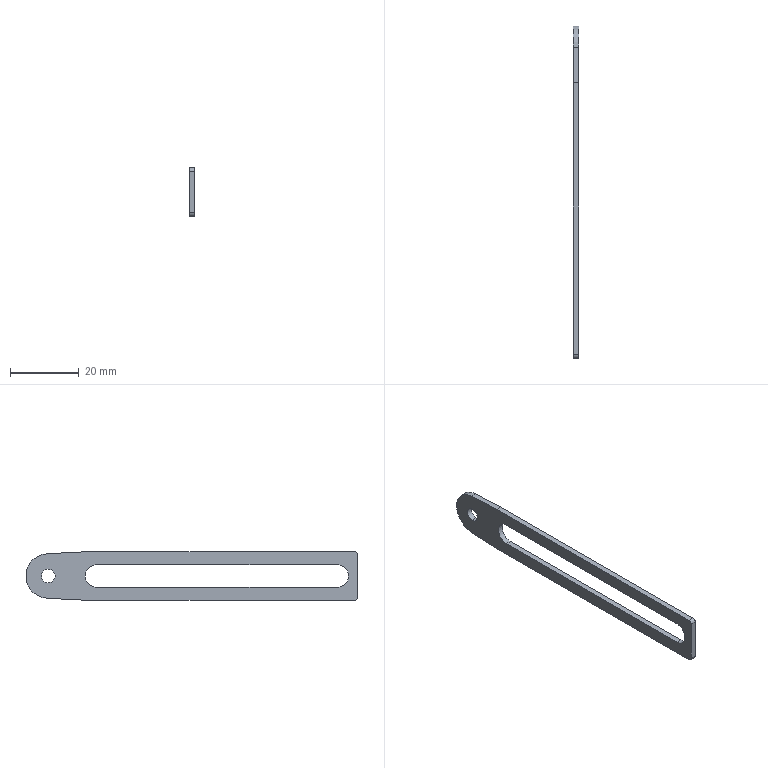Part | STEP file | Guide wheel mechanism revised.sldasm-Part-508 | 1 solid | 16 faces | box 1.6 x 96.5 x 14 mm | volume 1312 mm3 | plane 9 | cylinder 7 | commonest cylinder face diameters 2 x2 4 x2 6.5 x2 13 x1
STEP:
#1=CARTESIAN_POINT('',(0.,84.,-2.));
#2=VERTEX_POINT('',#1);
#3=CARTESIAN_POINT('',(0.,84.,2.));
#4=VERTEX_POINT('',#3);
#5=CARTESIAN_POINT('',(0.,84.,0.));
#6=DIRECTION('',(-1.,0.,0.));
#7=DIRECTION('',(0.,0.,-1.));
#8=AXIS2_PLACEMENT_3D('',#5,#6,#7);
#9=CIRCLE('',#8,2.);
#10=EDGE_CURVE('',#2,#4,#9,.T.);
#11=ORIENTED_EDGE('',*,*,#10,.T.);
#12=CARTESIAN_POINT('',(1.6,84.,2.));
#13=VERTEX_POINT('',#12);
#14=CARTESIAN_POINT('',(0.,84.,2.));
#15=DIRECTION('',(1.,0.,0.));
#16=VECTOR('',#15,1000.);
#17=LINE('',#14,#16);
#18=EDGE_CURVE('',#4,#13,#17,.T.);
#19=ORIENTED_EDGE('',*,*,#18,.T.);
#20=CARTESIAN_POINT('',(1.6,84.,-2.));
#21=VERTEX_POINT('',#20);
#22=CARTESIAN_POINT('',(1.6,84.,0.));
#23=DIRECTION('',(-1.,0.,0.));
#24=DIRECTION('',(0.,0.,-1.));
#25=AXIS2_PLACEMENT_3D('',#22,#23,#24);
#26=CIRCLE('',#25,2.);
#27=EDGE_CURVE('',#21,#13,#26,.T.);
#28=ORIENTED_EDGE('',*,*,#27,.F.);
#29=CARTESIAN_POINT('',(0.,84.,-2.));
#30=DIRECTION('',(1.,0.,0.));
#31=VECTOR('',#30,1000.);
#32=LINE('',#29,#31);
#33=EDGE_CURVE('',#2,#21,#32,.T.);
#34=ORIENTED_EDGE('',*,*,#33,.F.);
#35=EDGE_LOOP('',(#11,#19,#28,#34));
#36=FACE_OUTER_BOUND('',#35,.T.);
#37=CARTESIAN_POINT('',(0.,84.,0.));
#38=DIRECTION('',(1.,0.,0.));
#39=DIRECTION('',(0.,0.,-1.));
#40=AXIS2_PLACEMENT_3D('',#37,#38,#39);
#41=CYLINDRICAL_SURFACE('',#40,2.);
#42=ADVANCED_FACE('',(#36),#41,.F.);
#43=CARTESIAN_POINT('',(0.,70.,-3.25));
#44=VERTEX_POINT('',#43);
#45=CARTESIAN_POINT('',(0.,0.,-3.25));
#46=VERTEX_POINT('',#45);
#47=CARTESIAN_POINT('',(0.,0.,-3.25));
#48=DIRECTION('',(0.,-1.,0.));
#49=VECTOR('',#48,1000.);
#50=LINE('',#47,#49);
#51=EDGE_CURVE('',#44,#46,#50,.T.);
#52=ORIENTED_EDGE('',*,*,#51,.F.);
#53=CARTESIAN_POINT('',(0.,70.,3.25));
#54=VERTEX_POINT('',#53);
#55=CARTESIAN_POINT('',(0.,70.,0.));
#56=DIRECTION('',(-1.,0.,0.));
#57=DIRECTION('',(0.,0.,-1.));
#58=AXIS2_PLACEMENT_3D('',#55,#56,#57);
#59=CIRCLE('',#58,3.25);
#60=EDGE_CURVE('',#54,#44,#59,.T.);
#61=ORIENTED_EDGE('',*,*,#60,.F.);
#62=CARTESIAN_POINT('',(0.,0.,3.25));
#63=VERTEX_POINT('',#62);
#64=CARTESIAN_POINT('',(0.,0.,3.25));
#65=DIRECTION('',(0.,1.,0.));
#66=VECTOR('',#65,1000.);
#67=LINE('',#64,#66);
#68=EDGE_CURVE('',#63,#54,#67,.T.);
#69=ORIENTED_EDGE('',*,*,#68,.F.);
#70=CARTESIAN_POINT('',(0.,0.,0.));
#71=DIRECTION('',(-1.,0.,0.));
#72=DIRECTION('',(0.,0.,-1.));
#73=AXIS2_PLACEMENT_3D('',#70,#71,#72);
#74=CIRCLE('',#73,3.25);
#75=EDGE_CURVE('',#46,#63,#74,.T.);
#76=ORIENTED_EDGE('',*,*,#75,.F.);
#77=EDGE_LOOP('',(#52,#61,#69,#76));
#78=FACE_BOUND('',#77,.T.);
#79=ORIENTED_EDGE('',*,*,#10,.F.);
#80=CARTESIAN_POINT('',(0.,84.,0.));
#81=DIRECTION('',(-1.,0.,0.));
#82=DIRECTION('',(0.,0.,-1.));
#83=AXIS2_PLACEMENT_3D('',#80,#81,#82);
#84=CIRCLE('',#83,2.);
#85=EDGE_CURVE('',#4,#2,#84,.T.);
#86=ORIENTED_EDGE('',*,*,#85,.F.);
#87=EDGE_LOOP('',(#79,#86));
#88=FACE_BOUND('',#87,.T.);
#89=CARTESIAN_POINT('',(0.,84.32,6.492));
#90=VERTEX_POINT('',#89);
#91=CARTESIAN_POINT('',(0.,74.,7.));
#92=VERTEX_POINT('',#91);
#93=CARTESIAN_POINT('',(0.,84.32,6.492));
#94=DIRECTION('',(0.,-0.9988,0.04915));
#95=VECTOR('',#94,1000.);
#96=LINE('',#93,#95);
#97=EDGE_CURVE('',#90,#92,#96,.T.);
#98=ORIENTED_EDGE('',*,*,#97,.F.);
#99=CARTESIAN_POINT('',(0.,84.32,-6.492));
#100=VERTEX_POINT('',#99);
#101=CARTESIAN_POINT('',(0.,84.,0.));
#102=DIRECTION('',(1.,0.,0.));
#103=DIRECTION('',(0.,0.,-1.));
#104=AXIS2_PLACEMENT_3D('',#101,#102,#103);
#105=CIRCLE('',#104,6.5);
#106=EDGE_CURVE('',#100,#90,#105,.T.);
#107=ORIENTED_EDGE('',*,*,#106,.F.);
#108=CARTESIAN_POINT('',(0.,74.,-7.));
#109=VERTEX_POINT('',#108);
#110=CARTESIAN_POINT('',(0.,74.,-7.));
#111=DIRECTION('',(0.,0.9988,0.04915));
#112=VECTOR('',#111,1000.);
#113=LINE('',#110,#112);
#114=EDGE_CURVE('',#109,#100,#113,.T.);
#115=ORIENTED_EDGE('',*,*,#114,.F.);
#116=CARTESIAN_POINT('',(0.,-5.,-7.));
#117=VERTEX_POINT('',#116);
#118=CARTESIAN_POINT('',(0.,0.,-7.));
#119=DIRECTION('',(0.,1.,0.));
#120=VECTOR('',#119,1000.);
#121=LINE('',#118,#120);
#122=EDGE_CURVE('',#117,#109,#121,.T.);
#123=ORIENTED_EDGE('',*,*,#122,.F.);
#124=CARTESIAN_POINT('',(0.,-6.,-6.));
#125=VERTEX_POINT('',#124);
#126=CARTESIAN_POINT('',(0.,-5.,-6.));
#127=DIRECTION('',(1.,0.,0.));
#128=DIRECTION('',(0.,0.,1.));
#129=AXIS2_PLACEMENT_3D('',#126,#127,#128);
#130=CIRCLE('',#129,1.);
#131=EDGE_CURVE('',#125,#117,#130,.T.);
#132=ORIENTED_EDGE('',*,*,#131,.F.);
#133=CARTESIAN_POINT('',(0.,-6.,6.));
#134=VERTEX_POINT('',#133);
#135=CARTESIAN_POINT('',(0.,-6.,0.));
#136=DIRECTION('',(0.,0.,-1.));
#137=VECTOR('',#136,1000.);
#138=LINE('',#135,#137);
#139=EDGE_CURVE('',#134,#125,#138,.T.);
#140=ORIENTED_EDGE('',*,*,#139,.F.);
#141=CARTESIAN_POINT('',(0.,-5.,7.));
#142=VERTEX_POINT('',#141);
#143=CARTESIAN_POINT('',(0.,-5.,6.));
#144=DIRECTION('',(1.,0.,0.));
#145=DIRECTION('',(0.,0.,1.));
#146=AXIS2_PLACEMENT_3D('',#143,#144,#145);
#147=CIRCLE('',#146,1.);
#148=EDGE_CURVE('',#142,#134,#147,.T.);
#149=ORIENTED_EDGE('',*,*,#148,.F.);
#150=CARTESIAN_POINT('',(0.,0.,7.));
#151=DIRECTION('',(0.,-1.,0.));
#152=VECTOR('',#151,1000.);
#153=LINE('',#150,#152);
#154=EDGE_CURVE('',#92,#142,#153,.T.);
#155=ORIENTED_EDGE('',*,*,#154,.F.);
#156=EDGE_LOOP('',(#98,#107,#115,#123,#132,#140,#149,#155));
#157=FACE_OUTER_BOUND('',#156,.T.);
#158=CARTESIAN_POINT('',(0.,0.,0.));
#159=DIRECTION('',(1.,0.,0.));
#160=DIRECTION('',(0.,0.,-1.));
#161=AXIS2_PLACEMENT_3D('',#158,#159,#160);
#162=PLANE('',#161);
#163=ADVANCED_FACE('',(#78,#88,#157),#162,.F.);
#164=CARTESIAN_POINT('',(1.6,0.,-3.25));
#165=VERTEX_POINT('',#164);
#166=CARTESIAN_POINT('',(1.6,0.,3.25));
#167=VERTEX_POINT('',#166);
#168=CARTESIAN_POINT('',(1.6,0.,0.));
#169=DIRECTION('',(-1.,0.,0.));
#170=DIRECTION('',(0.,0.,-1.));
#171=AXIS2_PLACEMENT_3D('',#168,#169,#170);
#172=CIRCLE('',#171,3.25);
#173=EDGE_CURVE('',#165,#167,#172,.T.);
#174=ORIENTED_EDGE('',*,*,#173,.F.);
#175=CARTESIAN_POINT('',(0.,0.,-3.25));
#176=DIRECTION('',(1.,0.,0.));
#177=VECTOR('',#176,1000.);
#178=LINE('',#175,#177);
#179=EDGE_CURVE('',#46,#165,#178,.T.);
#180=ORIENTED_EDGE('',*,*,#179,.F.);
#181=ORIENTED_EDGE('',*,*,#75,.T.);
#182=CARTESIAN_POINT('',(0.,0.,3.25));
#183=DIRECTION('',(-1.,0.,0.));
#184=VECTOR('',#183,1000.);
#185=LINE('',#182,#184);
#186=EDGE_CURVE('',#167,#63,#185,.T.);
#187=ORIENTED_EDGE('',*,*,#186,.F.);
#188=EDGE_LOOP('',(#174,#180,#181,#187));
#189=FACE_OUTER_BOUND('',#188,.T.);
#190=CARTESIAN_POINT('',(0.,0.,0.));
#191=DIRECTION('',(1.,0.,0.));
#192=DIRECTION('',(0.,0.,-1.));
#193=AXIS2_PLACEMENT_3D('',#190,#191,#192);
#194=CYLINDRICAL_SURFACE('',#193,3.25);
#195=ADVANCED_FACE('',(#189),#194,.F.);
#196=CARTESIAN_POINT('',(1.6,70.,-3.25));
#197=VERTEX_POINT('',#196);
#198=CARTESIAN_POINT('',(0.,70.,-3.25));
#199=DIRECTION('',(-1.,0.,0.));
#200=VECTOR('',#199,1000.);
#201=LINE('',#198,#200);
#202=EDGE_CURVE('',#197,#44,#201,.T.);
#203=ORIENTED_EDGE('',*,*,#202,.T.);
#204=ORIENTED_EDGE('',*,*,#51,.T.);
#205=ORIENTED_EDGE('',*,*,#179,.T.);
#206=CARTESIAN_POINT('',(1.6,70.,-3.25));
#207=DIRECTION('',(0.,1.,0.));
#208=VECTOR('',#207,1000.);
#209=LINE('',#206,#208);
#210=EDGE_CURVE('',#165,#197,#209,.T.);
#211=ORIENTED_EDGE('',*,*,#210,.T.);
#212=EDGE_LOOP('',(#203,#204,#205,#211));
#213=FACE_OUTER_BOUND('',#212,.T.);
#214=CARTESIAN_POINT('',(0.,70.,-3.25));
#215=DIRECTION('',(0.,0.,1.));
#216=DIRECTION('',(0.,-1.,0.));
#217=AXIS2_PLACEMENT_3D('',#214,#215,#216);
#218=PLANE('',#217);
#219=ADVANCED_FACE('',(#213),#218,.T.);
#220=CARTESIAN_POINT('',(1.6,70.,3.25));
#221=VERTEX_POINT('',#220);
#222=CARTESIAN_POINT('',(1.6,70.,0.));
#223=DIRECTION('',(-1.,0.,0.));
#224=DIRECTION('',(0.,0.,-1.));
#225=AXIS2_PLACEMENT_3D('',#222,#223,#224);
#226=CIRCLE('',#225,3.25);
#227=EDGE_CURVE('',#221,#197,#226,.T.);
#228=ORIENTED_EDGE('',*,*,#227,.F.);
#229=CARTESIAN_POINT('',(0.,70.,3.25));
#230=DIRECTION('',(1.,0.,0.));
#231=VECTOR('',#230,1000.);
#232=LINE('',#229,#231);
#233=EDGE_CURVE('',#54,#221,#232,.T.);
#234=ORIENTED_EDGE('',*,*,#233,.F.);
#235=ORIENTED_EDGE('',*,*,#60,.T.);
#236=ORIENTED_EDGE('',*,*,#202,.F.);
#237=EDGE_LOOP('',(#228,#234,#235,#236));
#238=FACE_OUTER_BOUND('',#237,.T.);
#239=CARTESIAN_POINT('',(0.,70.,0.));
#240=DIRECTION('',(1.,0.,0.));
#241=DIRECTION('',(0.,0.,-1.));
#242=AXIS2_PLACEMENT_3D('',#239,#240,#241);
#243=CYLINDRICAL_SURFACE('',#242,3.25);
#244=ADVANCED_FACE('',(#238),#243,.F.);
#245=ORIENTED_EDGE('',*,*,#186,.T.);
#246=ORIENTED_EDGE('',*,*,#68,.T.);
#247=ORIENTED_EDGE('',*,*,#233,.T.);
#248=CARTESIAN_POINT('',(1.6,0.,3.25));
#249=DIRECTION('',(0.,-1.,0.));
#250=VECTOR('',#249,1000.);
#251=LINE('',#248,#250);
#252=EDGE_CURVE('',#221,#167,#251,.T.);
#253=ORIENTED_EDGE('',*,*,#252,.T.);
#254=EDGE_LOOP('',(#245,#246,#247,#253));
#255=FACE_OUTER_BOUND('',#254,.T.);
#256=CARTESIAN_POINT('',(0.,0.,3.25));
#257=DIRECTION('',(0.,0.,-1.));
#258=DIRECTION('',(0.,1.,0.));
#259=AXIS2_PLACEMENT_3D('',#256,#257,#258);
#260=PLANE('',#259);
#261=ADVANCED_FACE('',(#255),#260,.T.);
#262=ORIENTED_EDGE('',*,*,#18,.F.);
#263=ORIENTED_EDGE('',*,*,#85,.T.);
#264=ORIENTED_EDGE('',*,*,#33,.T.);
#265=CARTESIAN_POINT('',(1.6,84.,0.));
#266=DIRECTION('',(-1.,0.,0.));
#267=DIRECTION('',(0.,0.,-1.));
#268=AXIS2_PLACEMENT_3D('',#265,#266,#267);
#269=CIRCLE('',#268,2.);
#270=EDGE_CURVE('',#13,#21,#269,.T.);
#271=ORIENTED_EDGE('',*,*,#270,.F.);
#272=EDGE_LOOP('',(#262,#263,#264,#271));
#273=FACE_OUTER_BOUND('',#272,.T.);
#274=CARTESIAN_POINT('',(0.,84.,0.));
#275=DIRECTION('',(1.,0.,0.));
#276=DIRECTION('',(0.,0.,-1.));
#277=AXIS2_PLACEMENT_3D('',#274,#275,#276);
#278=CYLINDRICAL_SURFACE('',#277,2.);
#279=ADVANCED_FACE('',(#273),#278,.F.);
#280=ORIENTED_EDGE('',*,*,#154,.T.);
#281=CARTESIAN_POINT('',(1.6,-5.,7.));
#282=VERTEX_POINT('',#281);
#283=CARTESIAN_POINT('',(0.,-5.,7.));
#284=DIRECTION('',(1.,0.,0.));
#285=VECTOR('',#284,1000.);
#286=LINE('',#283,#285);
#287=EDGE_CURVE('',#142,#282,#286,.T.);
#288=ORIENTED_EDGE('',*,*,#287,.T.);
#289=CARTESIAN_POINT('',(1.6,74.,7.));
#290=VERTEX_POINT('',#289);
#291=CARTESIAN_POINT('',(1.6,74.,7.));
#292=DIRECTION('',(0.,1.,0.));
#293=VECTOR('',#292,1000.);
#294=LINE('',#291,#293);
#295=EDGE_CURVE('',#282,#290,#294,.T.);
#296=ORIENTED_EDGE('',*,*,#295,.T.);
#297=CARTESIAN_POINT('',(0.,74.,7.));
#298=DIRECTION('',(-1.,0.,0.));
#299=VECTOR('',#298,1000.);
#300=LINE('',#297,#299);
#301=EDGE_CURVE('',#290,#92,#300,.T.);
#302=ORIENTED_EDGE('',*,*,#301,.T.);
#303=EDGE_LOOP('',(#280,#288,#296,#302));
#304=FACE_OUTER_BOUND('',#303,.T.);
#305=CARTESIAN_POINT('',(0.,74.,7.));
#306=DIRECTION('',(0.,0.,1.));
#307=DIRECTION('',(1.,0.,0.));
#308=AXIS2_PLACEMENT_3D('',#305,#306,#307);
#309=PLANE('',#308);
#310=ADVANCED_FACE('',(#304),#309,.T.);
#311=CARTESIAN_POINT('',(1.6,84.32,6.492));
#312=VERTEX_POINT('',#311);
#313=CARTESIAN_POINT('',(0.,84.32,6.492));
#314=DIRECTION('',(-1.,0.,0.));
#315=VECTOR('',#314,1000.);
#316=LINE('',#313,#315);
#317=EDGE_CURVE('',#312,#90,#316,.T.);
#318=ORIENTED_EDGE('',*,*,#317,.T.);
#319=ORIENTED_EDGE('',*,*,#97,.T.);
#320=ORIENTED_EDGE('',*,*,#301,.F.);
#321=CARTESIAN_POINT('',(1.6,84.32,6.492));
#322=DIRECTION('',(0.,0.9988,-0.04915));
#323=VECTOR('',#322,1000.);
#324=LINE('',#321,#323);
#325=EDGE_CURVE('',#290,#312,#324,.T.);
#326=ORIENTED_EDGE('',*,*,#325,.T.);
#327=EDGE_LOOP('',(#318,#319,#320,#326));
#328=FACE_OUTER_BOUND('',#327,.T.);
#329=CARTESIAN_POINT('',(0.,84.32,6.492));
#330=DIRECTION('',(0.,0.04915,0.9988));
#331=DIRECTION('',(0.,-0.9988,0.04915));
#332=AXIS2_PLACEMENT_3D('',#329,#330,#331);
#333=PLANE('',#332);
#334=ADVANCED_FACE('',(#328),#333,.T.);
#335=CARTESIAN_POINT('',(1.6,84.32,-6.492));
#336=VERTEX_POINT('',#335);
#337=CARTESIAN_POINT('',(0.,84.32,-6.492));
#338=DIRECTION('',(-1.,0.,0.));
#339=VECTOR('',#338,1000.);
#340=LINE('',#337,#339);
#341=EDGE_CURVE('',#336,#100,#340,.T.);
#342=ORIENTED_EDGE('',*,*,#341,.T.);
#343=ORIENTED_EDGE('',*,*,#106,.T.);
#344=ORIENTED_EDGE('',*,*,#317,.F.);
#345=CARTESIAN_POINT('',(1.6,84.,0.));
#346=DIRECTION('',(-1.,0.,0.));
#347=DIRECTION('',(0.,0.,-1.));
#348=AXIS2_PLACEMENT_3D('',#345,#346,#347);
#349=CIRCLE('',#348,6.5);
#350=EDGE_CURVE('',#312,#336,#349,.T.);
#351=ORIENTED_EDGE('',*,*,#350,.T.);
#352=EDGE_LOOP('',(#342,#343,#344,#351));
#353=FACE_OUTER_BOUND('',#352,.T.);
#354=CARTESIAN_POINT('',(0.,84.,0.));
#355=DIRECTION('',(1.,0.,0.));
#356=DIRECTION('',(0.,0.,-1.));
#357=AXIS2_PLACEMENT_3D('',#354,#355,#356);
#358=CYLINDRICAL_SURFACE('',#357,6.5);
#359=ADVANCED_FACE('',(#353),#358,.T.);
#360=CARTESIAN_POINT('',(1.6,74.,-7.));
#361=VERTEX_POINT('',#360);
#362=CARTESIAN_POINT('',(0.,74.,-7.));
#363=DIRECTION('',(-1.,0.,0.));
#364=VECTOR('',#363,1000.);
#365=LINE('',#362,#364);
#366=EDGE_CURVE('',#361,#109,#365,.T.);
#367=ORIENTED_EDGE('',*,*,#366,.T.);
#368=ORIENTED_EDGE('',*,*,#114,.T.);
#369=ORIENTED_EDGE('',*,*,#341,.F.);
#370=CARTESIAN_POINT('',(1.6,74.,-7.));
#371=DIRECTION('',(0.,-0.9988,-0.04915));
#372=VECTOR('',#371,1000.);
#373=LINE('',#370,#372);
#374=EDGE_CURVE('',#336,#361,#373,.T.);
#375=ORIENTED_EDGE('',*,*,#374,.T.);
#376=EDGE_LOOP('',(#367,#368,#369,#375));
#377=FACE_OUTER_BOUND('',#376,.T.);
#378=CARTESIAN_POINT('',(0.,74.,-7.));
#379=DIRECTION('',(0.,0.04915,-0.9988));
#380=DIRECTION('',(0.,0.9988,0.04915));
#381=AXIS2_PLACEMENT_3D('',#378,#379,#380);
#382=PLANE('',#381);
#383=ADVANCED_FACE('',(#377),#382,.T.);
#384=CARTESIAN_POINT('',(1.6,-5.,-7.));
#385=VERTEX_POINT('',#384);
#386=CARTESIAN_POINT('',(1.6,-6.,-7.));
#387=DIRECTION('',(0.,-1.,0.));
#388=VECTOR('',#387,1000.);
#389=LINE('',#386,#388);
#390=EDGE_CURVE('',#361,#385,#389,.T.);
#391=ORIENTED_EDGE('',*,*,#390,.T.);
#392=CARTESIAN_POINT('',(0.,-5.,-7.));
#393=DIRECTION('',(-1.,0.,0.));
#394=VECTOR('',#393,1000.);
#395=LINE('',#392,#394);
#396=EDGE_CURVE('',#385,#117,#395,.T.);
#397=ORIENTED_EDGE('',*,*,#396,.T.);
#398=ORIENTED_EDGE('',*,*,#122,.T.);
#399=ORIENTED_EDGE('',*,*,#366,.F.);
#400=EDGE_LOOP('',(#391,#397,#398,#399));
#401=FACE_OUTER_BOUND('',#400,.T.);
#402=CARTESIAN_POINT('',(0.,-6.,-7.));
#403=DIRECTION('',(0.,0.,-1.));
#404=DIRECTION('',(-1.,0.,0.));
#405=AXIS2_PLACEMENT_3D('',#402,#403,#404);
#406=PLANE('',#405);
#407=ADVANCED_FACE('',(#401),#406,.T.);
#408=CARTESIAN_POINT('',(1.6,-6.,-6.));
#409=VERTEX_POINT('',#408);
#410=CARTESIAN_POINT('',(1.613,-6.,-6.));
#411=DIRECTION('',(-1.,0.,0.));
#412=VECTOR('',#411,1000.);
#413=LINE('',#410,#412);
#414=EDGE_CURVE('',#409,#125,#413,.T.);
#415=ORIENTED_EDGE('',*,*,#414,.T.);
#416=ORIENTED_EDGE('',*,*,#131,.T.);
#417=ORIENTED_EDGE('',*,*,#396,.F.);
#418=CARTESIAN_POINT('',(1.6,-5.,-6.));
#419=DIRECTION('',(-1.,0.,0.));
#420=DIRECTION('',(0.,0.,1.));
#421=AXIS2_PLACEMENT_3D('',#418,#419,#420);
#422=CIRCLE('',#421,1.);
#423=EDGE_CURVE('',#385,#409,#422,.T.);
#424=ORIENTED_EDGE('',*,*,#423,.T.);
#425=EDGE_LOOP('',(#415,#416,#417,#424));
#426=FACE_OUTER_BOUND('',#425,.T.);
#427=CARTESIAN_POINT('',(1.613,-5.,-6.));
#428=DIRECTION('',(-1.,0.,0.));
#429=DIRECTION('',(0.,0.,1.));
#430=AXIS2_PLACEMENT_3D('',#427,#428,#429);
#431=CYLINDRICAL_SURFACE('',#430,1.);
#432=ADVANCED_FACE('',(#426),#431,.T.);
#433=CARTESIAN_POINT('',(1.6,-6.,6.));
#434=VERTEX_POINT('',#433);
#435=CARTESIAN_POINT('',(1.6,-6.,7.));
#436=DIRECTION('',(0.,0.,1.));
#437=VECTOR('',#436,1000.);
#438=LINE('',#435,#437);
#439=EDGE_CURVE('',#409,#434,#438,.T.);
#440=ORIENTED_EDGE('',*,*,#439,.T.);
#441=CARTESIAN_POINT('',(0.,-6.,6.));
#442=DIRECTION('',(-1.,0.,0.));
#443=VECTOR('',#442,1000.);
#444=LINE('',#441,#443);
#445=EDGE_CURVE('',#434,#134,#444,.T.);
#446=ORIENTED_EDGE('',*,*,#445,.T.);
#447=ORIENTED_EDGE('',*,*,#139,.T.);
#448=ORIENTED_EDGE('',*,*,#414,.F.);
#449=EDGE_LOOP('',(#440,#446,#447,#448));
#450=FACE_OUTER_BOUND('',#449,.T.);
#451=CARTESIAN_POINT('',(0.,-6.,7.));
#452=DIRECTION('',(0.,-1.,0.));
#453=DIRECTION('',(0.,0.,-1.));
#454=AXIS2_PLACEMENT_3D('',#451,#452,#453);
#455=PLANE('',#454);
#456=ADVANCED_FACE('',(#450),#455,.T.);
#457=ORIENTED_EDGE('',*,*,#287,.F.);
#458=ORIENTED_EDGE('',*,*,#148,.T.);
#459=ORIENTED_EDGE('',*,*,#445,.F.);
#460=CARTESIAN_POINT('',(1.6,-5.,6.));
#461=DIRECTION('',(-1.,0.,0.));
#462=DIRECTION('',(0.,0.,1.));
#463=AXIS2_PLACEMENT_3D('',#460,#461,#462);
#464=CIRCLE('',#463,1.);
#465=EDGE_CURVE('',#434,#282,#464,.T.);
#466=ORIENTED_EDGE('',*,*,#465,.T.);
#467=EDGE_LOOP('',(#457,#458,#459,#466));
#468=FACE_OUTER_BOUND('',#467,.T.);
#469=CARTESIAN_POINT('',(1.613,-5.,6.));
#470=DIRECTION('',(-1.,0.,0.));
#471=DIRECTION('',(0.,0.,1.));
#472=AXIS2_PLACEMENT_3D('',#469,#470,#471);
#473=CYLINDRICAL_SURFACE('',#472,1.);
#474=ADVANCED_FACE('',(#468),#473,.T.);
#475=ORIENTED_EDGE('',*,*,#173,.T.);
#476=ORIENTED_EDGE('',*,*,#252,.F.);
#477=ORIENTED_EDGE('',*,*,#227,.T.);
#478=ORIENTED_EDGE('',*,*,#210,.F.);
#479=EDGE_LOOP('',(#475,#476,#477,#478));
#480=FACE_BOUND('',#479,.T.);
#481=ORIENTED_EDGE('',*,*,#27,.T.);
#482=ORIENTED_EDGE('',*,*,#270,.T.);
#483=EDGE_LOOP('',(#481,#482));
#484=FACE_BOUND('',#483,.T.);
#485=ORIENTED_EDGE('',*,*,#295,.F.);
#486=ORIENTED_EDGE('',*,*,#465,.F.);
#487=ORIENTED_EDGE('',*,*,#439,.F.);
#488=ORIENTED_EDGE('',*,*,#423,.F.);
#489=ORIENTED_EDGE('',*,*,#390,.F.);
#490=ORIENTED_EDGE('',*,*,#374,.F.);
#491=ORIENTED_EDGE('',*,*,#350,.F.);
#492=ORIENTED_EDGE('',*,*,#325,.F.);
#493=EDGE_LOOP('',(#485,#486,#487,#488,#489,#490,#491,#492));
#494=FACE_OUTER_BOUND('',#493,.T.);
#495=CARTESIAN_POINT('',(1.6,0.,0.));
#496=DIRECTION('',(1.,0.,0.));
#497=DIRECTION('',(0.,0.,-1.));
#498=AXIS2_PLACEMENT_3D('',#495,#496,#497);
#499=PLANE('',#498);
#500=ADVANCED_FACE('',(#480,#484,#494),#499,.T.);
#501=CLOSED_SHELL('',(#42,#163,#195,#219,#244,#261,#279,#310,#334,#359,#383,#407,#432,#456,#474,#500));
#502=MANIFOLD_SOLID_BREP('',#501);
#503=CARTESIAN_POINT('',(0.,0.,0.));
#504=DIRECTION('',(0.,0.,1.));
#505=DIRECTION('',(1.,0.,0.));
#506=AXIS2_PLACEMENT_3D('',#503,#504,#505);
#507=(LENGTH_UNIT()NAMED_UNIT(*)SI_UNIT(.MILLI.,.METRE.));
#508=UNCERTAINTY_MEASURE_WITH_UNIT(LENGTH_MEASURE(0.00001),#507,'','');
#509=(NAMED_UNIT(*)PLANE_ANGLE_UNIT()SI_UNIT($,.RADIAN.));
#510=(NAMED_UNIT(*)SI_UNIT($,.STERADIAN.)SOLID_ANGLE_UNIT());
#511=(GEOMETRIC_REPRESENTATION_CONTEXT(3)GLOBAL_UNCERTAINTY_ASSIGNED_CONTEXT((#508))GLOBAL_UNIT_ASSIGNED_CONTEXT((#507,#509,#510))REPRESENTATION_CONTEXT('',''));
#512=ADVANCED_BREP_SHAPE_REPRESENTATION('',(#502,#506),#511);